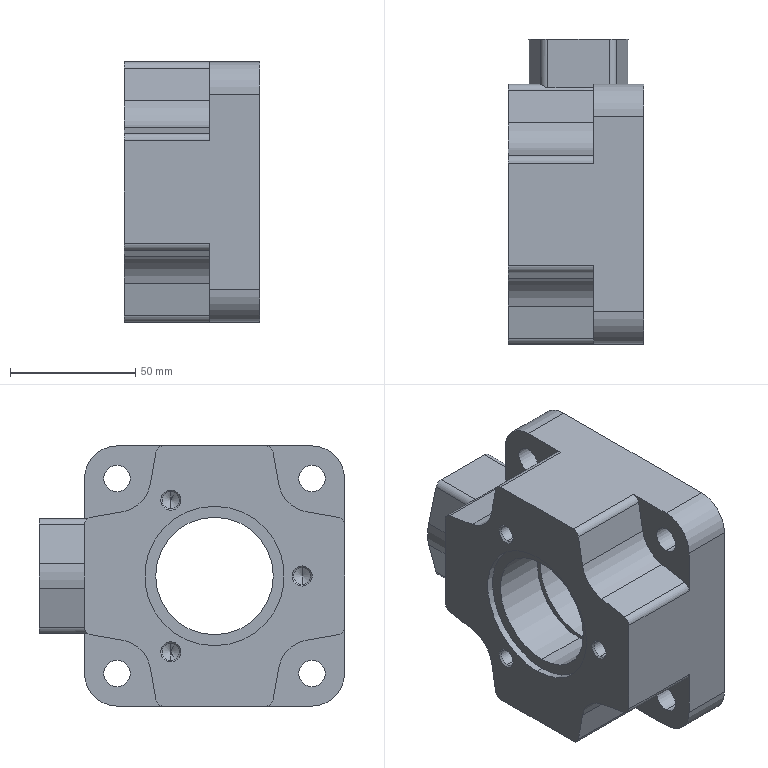Part | SolidWorks | features ICE 11, HoleWzd 3, Chamfer 2, Extrusion 1, Fillet 1 | 1 solid | 122 faces | box 54 x 122 x 104 mm | volume 319990 mm3 | cylinder 56 | plane 33 | cone 26 | torus 6 | spline 1 | commonest cylinder face diameters 6 x12 10.5 x8 6.8 x6 26 x4 27 x4 47 x4